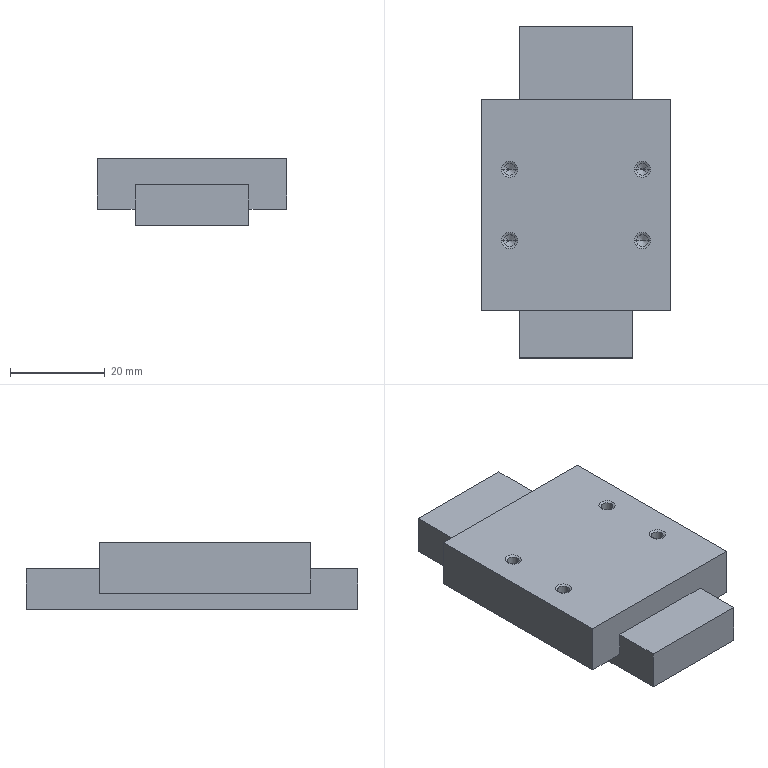Part | NX | 1 solid | 44 faces | box 40 x 70 x 14 mm | volume 27390 mm3 | plane 16 | cone 16 | cylinder 12 | commonest cylinder face diameters 2.5 x8 4.5 x4
STEP:
#1=CARTESIAN_POINT('',(521.985,-261.815,-57.349));
#2=VERTEX_POINT('',#1);
#3=CARTESIAN_POINT('',(526.485,-261.817,-57.349));
#4=VERTEX_POINT('',#3);
#5=CARTESIAN_POINT('',(524.235,-261.816,-57.349));
#6=DIRECTION('',(0.,0.,1.));
#7=DIRECTION('',(1.,-0.0003046,0.));
#8=AXIS2_PLACEMENT_3D('',#5,#6,#7);
#9=CIRCLE('',#8,2.25);
#10=EDGE_CURVE('',#2,#4,#9,.T.);
#11=ORIENTED_EDGE('',*,*,#10,.F.);
#12=CARTESIAN_POINT('',(524.235,-261.816,-57.349));
#13=DIRECTION('',(0.,0.,1.));
#14=DIRECTION('',(1.,-0.0003046,0.));
#15=AXIS2_PLACEMENT_3D('',#12,#13,#14);
#16=CIRCLE('',#15,2.25);
#17=EDGE_CURVE('',#4,#2,#16,.T.);
#18=ORIENTED_EDGE('',*,*,#17,.F.);
#19=EDGE_LOOP('',(#11,#18));
#20=FACE_BOUND('',#19,.T.);
#21=CARTESIAN_POINT('',(520.86,-261.832,-57.349));
#22=DIRECTION('',(0.,0.,1.));
#23=DIRECTION('',(1.,0.,0.));
#24=AXIS2_PLACEMENT_3D('',#21,#22,#23);
#25=PLANE('',#24);
#26=ADVANCED_FACE('',(#20),#25,.F.);
#27=CARTESIAN_POINT('',(536.235,-316.816,-61.349));
#28=VERTEX_POINT('',#27);
#29=CARTESIAN_POINT('',(536.235,-246.816,-61.349));
#30=VERTEX_POINT('',#29);
#31=CARTESIAN_POINT('',(536.235,0.,-61.349));
#32=DIRECTION('',(0.,1.,0.));
#33=VECTOR('',#32,1000.);
#34=LINE('',#31,#33);
#35=EDGE_CURVE('',#28,#30,#34,.T.);
#36=ORIENTED_EDGE('',*,*,#35,.T.);
#37=CARTESIAN_POINT('',(536.235,-246.816,-52.849));
#38=VERTEX_POINT('',#37);
#39=CARTESIAN_POINT('',(536.235,-246.816,0.));
#40=DIRECTION('',(0.,0.,1.));
#41=VECTOR('',#40,1000.);
#42=LINE('',#39,#41);
#43=EDGE_CURVE('',#30,#38,#42,.T.);
#44=ORIENTED_EDGE('',*,*,#43,.T.);
#45=CARTESIAN_POINT('',(536.235,-262.316,-52.849));
#46=VERTEX_POINT('',#45);
#47=CARTESIAN_POINT('',(536.235,0.,-52.849));
#48=DIRECTION('',(0.,1.,0.));
#49=VECTOR('',#48,1000.);
#50=LINE('',#47,#49);
#51=EDGE_CURVE('',#46,#38,#50,.T.);
#52=ORIENTED_EDGE('',*,*,#51,.F.);
#53=CARTESIAN_POINT('',(536.235,-262.316,-57.949));
#54=VERTEX_POINT('',#53);
#55=CARTESIAN_POINT('',(536.235,-262.316,0.));
#56=DIRECTION('',(0.,0.,1.));
#57=VECTOR('',#56,1000.);
#58=LINE('',#55,#57);
#59=EDGE_CURVE('',#54,#46,#58,.T.);
#60=ORIENTED_EDGE('',*,*,#59,.F.);
#61=CARTESIAN_POINT('',(536.235,-306.816,-57.949));
#62=VERTEX_POINT('',#61);
#63=CARTESIAN_POINT('',(536.235,0.,-57.949));
#64=DIRECTION('',(0.,-1.,0.));
#65=VECTOR('',#64,1000.);
#66=LINE('',#63,#65);
#67=EDGE_CURVE('',#54,#62,#66,.T.);
#68=ORIENTED_EDGE('',*,*,#67,.T.);
#69=CARTESIAN_POINT('',(536.235,-306.816,-52.849));
#70=VERTEX_POINT('',#69);
#71=CARTESIAN_POINT('',(536.235,-306.816,0.));
#72=DIRECTION('',(0.,0.,1.));
#73=VECTOR('',#72,1000.);
#74=LINE('',#71,#73);
#75=EDGE_CURVE('',#62,#70,#74,.T.);
#76=ORIENTED_EDGE('',*,*,#75,.T.);
#77=CARTESIAN_POINT('',(536.235,-316.816,-52.849));
#78=VERTEX_POINT('',#77);
#79=CARTESIAN_POINT('',(536.235,0.,-52.849));
#80=DIRECTION('',(0.,1.,0.));
#81=VECTOR('',#80,1000.);
#82=LINE('',#79,#81);
#83=EDGE_CURVE('',#78,#70,#82,.T.);
#84=ORIENTED_EDGE('',*,*,#83,.F.);
#85=CARTESIAN_POINT('',(536.235,-316.816,0.));
#86=DIRECTION('',(0.,0.,-1.));
#87=VECTOR('',#86,1000.);
#88=LINE('',#85,#87);
#89=EDGE_CURVE('',#78,#28,#88,.T.);
#90=ORIENTED_EDGE('',*,*,#89,.T.);
#91=EDGE_LOOP('',(#36,#44,#52,#60,#68,#76,#84,#90));
#92=FACE_BOUND('',#91,.T.);
#93=CARTESIAN_POINT('',(536.235,-306.816,-52.849));
#94=DIRECTION('',(-1.,0.,0.));
#95=DIRECTION('',(0.,1.,0.));
#96=AXIS2_PLACEMENT_3D('',#93,#94,#95);
#97=PLANE('',#96);
#98=ADVANCED_FACE('',(#92),#97,.F.);
#99=CARTESIAN_POINT('',(544.235,-262.316,-47.349));
#100=VERTEX_POINT('',#99);
#101=CARTESIAN_POINT('',(544.235,-306.816,-47.349));
#102=VERTEX_POINT('',#101);
#103=CARTESIAN_POINT('',(544.235,0.,-47.349));
#104=DIRECTION('',(0.,-1.,0.));
#105=VECTOR('',#104,1000.);
#106=LINE('',#103,#105);
#107=EDGE_CURVE('',#100,#102,#106,.T.);
#108=ORIENTED_EDGE('',*,*,#107,.F.);
#109=CARTESIAN_POINT('',(504.235,-262.316,-47.349));
#110=VERTEX_POINT('',#109);
#111=CARTESIAN_POINT('',(0.,-262.316,-47.349));
#112=DIRECTION('',(1.,0.,0.));
#113=VECTOR('',#112,1000.);
#114=LINE('',#111,#113);
#115=EDGE_CURVE('',#110,#100,#114,.T.);
#116=ORIENTED_EDGE('',*,*,#115,.F.);
#117=CARTESIAN_POINT('',(504.235,-306.816,-47.349));
#118=VERTEX_POINT('',#117);
#119=CARTESIAN_POINT('',(504.235,0.,-47.349));
#120=DIRECTION('',(0.,1.,0.));
#121=VECTOR('',#120,1000.);
#122=LINE('',#119,#121);
#123=EDGE_CURVE('',#118,#110,#122,.T.);
#124=ORIENTED_EDGE('',*,*,#123,.F.);
#125=CARTESIAN_POINT('',(0.,-306.816,-47.349));
#126=DIRECTION('',(-1.,0.,0.));
#127=VECTOR('',#126,1000.);
#128=LINE('',#125,#127);
#129=EDGE_CURVE('',#102,#118,#128,.T.);
#130=ORIENTED_EDGE('',*,*,#129,.F.);
#131=EDGE_LOOP('',(#108,#116,#124,#130));
#132=FACE_BOUND('',#131,.T.);
#133=CARTESIAN_POINT('',(511.935,-277.066,-47.349));
#134=VERTEX_POINT('',#133);
#135=CARTESIAN_POINT('',(508.535,-277.066,-47.349));
#136=VERTEX_POINT('',#135);
#137=CARTESIAN_POINT('',(510.235,-277.066,-47.349));
#138=DIRECTION('',(0.,0.,1.));
#139=DIRECTION('',(1.,0.,0.));
#140=AXIS2_PLACEMENT_3D('',#137,#138,#139);
#141=CIRCLE('',#140,1.7);
#142=EDGE_CURVE('',#134,#136,#141,.T.);
#143=ORIENTED_EDGE('',*,*,#142,.F.);
#144=CARTESIAN_POINT('',(510.235,-277.066,-47.349));
#145=DIRECTION('',(0.,0.,1.));
#146=DIRECTION('',(1.,0.,0.));
#147=AXIS2_PLACEMENT_3D('',#144,#145,#146);
#148=CIRCLE('',#147,1.7);
#149=EDGE_CURVE('',#136,#134,#148,.T.);
#150=ORIENTED_EDGE('',*,*,#149,.F.);
#151=EDGE_LOOP('',(#143,#150));
#152=FACE_BOUND('',#151,.T.);
#153=CARTESIAN_POINT('',(539.935,-277.066,-47.349));
#154=VERTEX_POINT('',#153);
#155=CARTESIAN_POINT('',(536.535,-277.066,-47.349));
#156=VERTEX_POINT('',#155);
#157=CARTESIAN_POINT('',(538.235,-277.066,-47.349));
#158=DIRECTION('',(0.,0.,1.));
#159=DIRECTION('',(1.,0.,0.));
#160=AXIS2_PLACEMENT_3D('',#157,#158,#159);
#161=CIRCLE('',#160,1.7);
#162=EDGE_CURVE('',#154,#156,#161,.T.);
#163=ORIENTED_EDGE('',*,*,#162,.F.);
#164=CARTESIAN_POINT('',(538.235,-277.066,-47.349));
#165=DIRECTION('',(0.,0.,1.));
#166=DIRECTION('',(1.,0.,0.));
#167=AXIS2_PLACEMENT_3D('',#164,#165,#166);
#168=CIRCLE('',#167,1.7);
#169=EDGE_CURVE('',#156,#154,#168,.T.);
#170=ORIENTED_EDGE('',*,*,#169,.F.);
#171=EDGE_LOOP('',(#163,#170));
#172=FACE_BOUND('',#171,.T.);
#173=CARTESIAN_POINT('',(508.535,-292.066,-47.349));
#174=VERTEX_POINT('',#173);
#175=CARTESIAN_POINT('',(511.935,-292.066,-47.349));
#176=VERTEX_POINT('',#175);
#177=CARTESIAN_POINT('',(510.235,-292.066,-47.349));
#178=DIRECTION('',(0.,0.,1.));
#179=DIRECTION('',(1.,0.,0.));
#180=AXIS2_PLACEMENT_3D('',#177,#178,#179);
#181=CIRCLE('',#180,1.7);
#182=EDGE_CURVE('',#174,#176,#181,.T.);
#183=ORIENTED_EDGE('',*,*,#182,.F.);
#184=CARTESIAN_POINT('',(510.235,-292.066,-47.349));
#185=DIRECTION('',(0.,0.,1.));
#186=DIRECTION('',(1.,0.,0.));
#187=AXIS2_PLACEMENT_3D('',#184,#185,#186);
#188=CIRCLE('',#187,1.7);
#189=EDGE_CURVE('',#176,#174,#188,.T.);
#190=ORIENTED_EDGE('',*,*,#189,.F.);
#191=EDGE_LOOP('',(#183,#190));
#192=FACE_BOUND('',#191,.T.);
#193=CARTESIAN_POINT('',(536.535,-292.066,-47.349));
#194=VERTEX_POINT('',#193);
#195=CARTESIAN_POINT('',(539.935,-292.066,-47.349));
#196=VERTEX_POINT('',#195);
#197=CARTESIAN_POINT('',(538.235,-292.066,-47.349));
#198=DIRECTION('',(0.,0.,1.));
#199=DIRECTION('',(1.,0.,0.));
#200=AXIS2_PLACEMENT_3D('',#197,#198,#199);
#201=CIRCLE('',#200,1.7);
#202=EDGE_CURVE('',#194,#196,#201,.T.);
#203=ORIENTED_EDGE('',*,*,#202,.F.);
#204=CARTESIAN_POINT('',(538.235,-292.066,-47.349));
#205=DIRECTION('',(0.,0.,1.));
#206=DIRECTION('',(1.,0.,0.));
#207=AXIS2_PLACEMENT_3D('',#204,#205,#206);
#208=CIRCLE('',#207,1.7);
#209=EDGE_CURVE('',#196,#194,#208,.T.);
#210=ORIENTED_EDGE('',*,*,#209,.F.);
#211=EDGE_LOOP('',(#203,#210));
#212=FACE_BOUND('',#211,.T.);
#213=CARTESIAN_POINT('',(504.235,-306.816,-47.349));
#214=DIRECTION('',(0.,0.,-1.));
#215=DIRECTION('',(-1.,0.,0.));
#216=AXIS2_PLACEMENT_3D('',#213,#214,#215);
#217=PLANE('',#216);
#218=ADVANCED_FACE('',(#132,#152,#172,#192,#212),#217,.F.);
#219=CARTESIAN_POINT('',(512.235,-316.816,-52.849));
#220=VERTEX_POINT('',#219);
#221=CARTESIAN_POINT('',(512.235,-306.816,-52.849));
#222=VERTEX_POINT('',#221);
#223=CARTESIAN_POINT('',(512.235,0.,-52.849));
#224=DIRECTION('',(0.,1.,0.));
#225=VECTOR('',#224,1000.);
#226=LINE('',#223,#225);
#227=EDGE_CURVE('',#220,#222,#226,.T.);
#228=ORIENTED_EDGE('',*,*,#227,.T.);
#229=CARTESIAN_POINT('',(512.235,-306.816,-57.949));
#230=VERTEX_POINT('',#229);
#231=CARTESIAN_POINT('',(512.235,-306.816,0.));
#232=DIRECTION('',(0.,0.,-1.));
#233=VECTOR('',#232,1000.);
#234=LINE('',#231,#233);
#235=EDGE_CURVE('',#222,#230,#234,.T.);
#236=ORIENTED_EDGE('',*,*,#235,.T.);
#237=CARTESIAN_POINT('',(512.235,-262.316,-57.949));
#238=VERTEX_POINT('',#237);
#239=CARTESIAN_POINT('',(512.235,0.,-57.949));
#240=DIRECTION('',(0.,1.,0.));
#241=VECTOR('',#240,1000.);
#242=LINE('',#239,#241);
#243=EDGE_CURVE('',#230,#238,#242,.T.);
#244=ORIENTED_EDGE('',*,*,#243,.T.);
#245=CARTESIAN_POINT('',(512.235,-262.316,-52.849));
#246=VERTEX_POINT('',#245);
#247=CARTESIAN_POINT('',(512.235,-262.316,0.));
#248=DIRECTION('',(0.,0.,-1.));
#249=VECTOR('',#248,1000.);
#250=LINE('',#247,#249);
#251=EDGE_CURVE('',#246,#238,#250,.T.);
#252=ORIENTED_EDGE('',*,*,#251,.F.);
#253=CARTESIAN_POINT('',(512.235,-246.816,-52.849));
#254=VERTEX_POINT('',#253);
#255=CARTESIAN_POINT('',(512.235,0.,-52.849));
#256=DIRECTION('',(0.,-1.,0.));
#257=VECTOR('',#256,1000.);
#258=LINE('',#255,#257);
#259=EDGE_CURVE('',#254,#246,#258,.T.);
#260=ORIENTED_EDGE('',*,*,#259,.F.);
#261=CARTESIAN_POINT('',(512.235,-246.816,-61.349));
#262=VERTEX_POINT('',#261);
#263=CARTESIAN_POINT('',(512.235,-246.816,0.));
#264=DIRECTION('',(0.,0.,-1.));
#265=VECTOR('',#264,1000.);
#266=LINE('',#263,#265);
#267=EDGE_CURVE('',#254,#262,#266,.T.);
#268=ORIENTED_EDGE('',*,*,#267,.T.);
#269=CARTESIAN_POINT('',(512.235,-316.816,-61.349));
#270=VERTEX_POINT('',#269);
#271=CARTESIAN_POINT('',(512.235,0.,-61.349));
#272=DIRECTION('',(0.,-1.,0.));
#273=VECTOR('',#272,1000.);
#274=LINE('',#271,#273);
#275=EDGE_CURVE('',#262,#270,#274,.T.);
#276=ORIENTED_EDGE('',*,*,#275,.T.);
#277=CARTESIAN_POINT('',(512.235,-316.816,0.));
#278=DIRECTION('',(0.,0.,1.));
#279=VECTOR('',#278,1000.);
#280=LINE('',#277,#279);
#281=EDGE_CURVE('',#270,#220,#280,.T.);
#282=ORIENTED_EDGE('',*,*,#281,.T.);
#283=EDGE_LOOP('',(#228,#236,#244,#252,#260,#268,#276,#282));
#284=FACE_BOUND('',#283,.T.);
#285=CARTESIAN_POINT('',(512.235,-306.816,-61.349));
#286=DIRECTION('',(1.,0.,0.));
#287=DIRECTION('',(0.,0.,-1.));
#288=AXIS2_PLACEMENT_3D('',#285,#286,#287);
#289=PLANE('',#288);
#290=ADVANCED_FACE('',(#284),#289,.F.);
#291=ORIENTED_EDGE('',*,*,#83,.T.);
#292=CARTESIAN_POINT('',(0.,-306.816,-52.849));
#293=DIRECTION('',(-1.,0.,0.));
#294=VECTOR('',#293,1000.);
#295=LINE('',#292,#294);
#296=EDGE_CURVE('',#70,#222,#295,.T.);
#297=ORIENTED_EDGE('',*,*,#296,.T.);
#298=ORIENTED_EDGE('',*,*,#227,.F.);
#299=CARTESIAN_POINT('',(0.,-316.816,-52.849));
#300=DIRECTION('',(1.,0.,0.));
#301=VECTOR('',#300,1000.);
#302=LINE('',#299,#301);
#303=EDGE_CURVE('',#220,#78,#302,.T.);
#304=ORIENTED_EDGE('',*,*,#303,.T.);
#305=EDGE_LOOP('',(#291,#297,#298,#304));
#306=FACE_BOUND('',#305,.T.);
#307=CARTESIAN_POINT('',(512.235,-306.816,-52.849));
#308=DIRECTION('',(0.,0.,-1.));
#309=DIRECTION('',(-1.,0.,0.));
#310=AXIS2_PLACEMENT_3D('',#307,#308,#309);
#311=PLANE('',#310);
#312=ADVANCED_FACE('',(#306),#311,.F.);
#313=ORIENTED_EDGE('',*,*,#67,.F.);
#314=CARTESIAN_POINT('',(544.235,-262.316,-57.949));
#315=VERTEX_POINT('',#314);
#316=CARTESIAN_POINT('',(0.,-262.316,-57.949));
#317=DIRECTION('',(1.,0.,0.));
#318=VECTOR('',#317,1000.);
#319=LINE('',#316,#318);
#320=EDGE_CURVE('',#54,#315,#319,.T.);
#321=ORIENTED_EDGE('',*,*,#320,.T.);
#322=CARTESIAN_POINT('',(544.235,-306.816,-57.949));
#323=VERTEX_POINT('',#322);
#324=CARTESIAN_POINT('',(544.235,0.,-57.949));
#325=DIRECTION('',(0.,1.,0.));
#326=VECTOR('',#325,1000.);
#327=LINE('',#324,#326);
#328=EDGE_CURVE('',#323,#315,#327,.T.);
#329=ORIENTED_EDGE('',*,*,#328,.F.);
#330=CARTESIAN_POINT('',(0.,-306.816,-57.949));
#331=DIRECTION('',(1.,0.,0.));
#332=VECTOR('',#331,1000.);
#333=LINE('',#330,#332);
#334=EDGE_CURVE('',#62,#323,#333,.T.);
#335=ORIENTED_EDGE('',*,*,#334,.F.);
#336=EDGE_LOOP('',(#313,#321,#329,#335));
#337=FACE_BOUND('',#336,.T.);
#338=CARTESIAN_POINT('',(544.235,-306.816,-57.949));
#339=DIRECTION('',(0.,0.,1.));
#340=DIRECTION('',(1.,0.,0.));
#341=AXIS2_PLACEMENT_3D('',#338,#339,#340);
#342=PLANE('',#341);
#343=ADVANCED_FACE('',(#337),#342,.F.);
#344=CARTESIAN_POINT('',(504.235,-262.316,-57.949));
#345=VERTEX_POINT('',#344);
#346=CARTESIAN_POINT('',(0.,-262.316,-57.949));
#347=DIRECTION('',(-1.,0.,0.));
#348=VECTOR('',#347,1000.);
#349=LINE('',#346,#348);
#350=EDGE_CURVE('',#238,#345,#349,.T.);
#351=ORIENTED_EDGE('',*,*,#350,.T.);
#352=CARTESIAN_POINT('',(504.235,-262.316,0.));
#353=DIRECTION('',(0.,0.,1.));
#354=VECTOR('',#353,1000.);
#355=LINE('',#352,#354);
#356=EDGE_CURVE('',#345,#110,#355,.T.);
#357=ORIENTED_EDGE('',*,*,#356,.T.);
#358=ORIENTED_EDGE('',*,*,#115,.T.);
#359=CARTESIAN_POINT('',(544.235,-262.316,0.));
#360=DIRECTION('',(0.,0.,-1.));
#361=VECTOR('',#360,1000.);
#362=LINE('',#359,#361);
#363=EDGE_CURVE('',#100,#315,#362,.T.);
#364=ORIENTED_EDGE('',*,*,#363,.T.);
#365=ORIENTED_EDGE('',*,*,#320,.F.);
#366=ORIENTED_EDGE('',*,*,#59,.T.);
#367=CARTESIAN_POINT('',(0.,-262.316,-52.849));
#368=DIRECTION('',(1.,0.,0.));
#369=VECTOR('',#368,1000.);
#370=LINE('',#367,#369);
#371=EDGE_CURVE('',#246,#46,#370,.T.);
#372=ORIENTED_EDGE('',*,*,#371,.F.);
#373=ORIENTED_EDGE('',*,*,#251,.T.);
#374=EDGE_LOOP('',(#351,#357,#358,#364,#365,#366,#372,#373));
#375=FACE_BOUND('',#374,.T.);
#376=CARTESIAN_POINT('',(492.609,-262.316,-65.209));
#377=DIRECTION('',(0.,1.,0.));
#378=DIRECTION('',(1.,0.,0.));
#379=AXIS2_PLACEMENT_3D('',#376,#377,#378);
#380=PLANE('',#379);
#381=ADVANCED_FACE('',(#375),#380,.T.);
#382=CARTESIAN_POINT('',(504.235,-306.816,-57.949));
#383=VERTEX_POINT('',#382);
#384=CARTESIAN_POINT('',(504.235,0.,-57.949));
#385=DIRECTION('',(0.,-1.,0.));
#386=VECTOR('',#385,1000.);
#387=LINE('',#384,#386);
#388=EDGE_CURVE('',#345,#383,#387,.T.);
#389=ORIENTED_EDGE('',*,*,#388,.F.);
#390=ORIENTED_EDGE('',*,*,#350,.F.);
#391=ORIENTED_EDGE('',*,*,#243,.F.);
#392=CARTESIAN_POINT('',(0.,-306.816,-57.949));
#393=DIRECTION('',(1.,0.,0.));
#394=VECTOR('',#393,1000.);
#395=LINE('',#392,#394);
#396=EDGE_CURVE('',#383,#230,#395,.T.);
#397=ORIENTED_EDGE('',*,*,#396,.F.);
#398=EDGE_LOOP('',(#389,#390,#391,#397));
#399=FACE_BOUND('',#398,.T.);
#400=CARTESIAN_POINT('',(512.235,-306.816,-57.949));
#401=DIRECTION('',(0.,0.,1.));
#402=DIRECTION('',(1.,0.,0.));
#403=AXIS2_PLACEMENT_3D('',#400,#401,#402);
#404=PLANE('',#403);
#405=ADVANCED_FACE('',(#399),#404,.F.);
#406=ORIENTED_EDGE('',*,*,#235,.F.);
#407=ORIENTED_EDGE('',*,*,#296,.F.);
#408=ORIENTED_EDGE('',*,*,#75,.F.);
#409=ORIENTED_EDGE('',*,*,#334,.T.);
#410=CARTESIAN_POINT('',(544.235,-306.816,0.));
#411=DIRECTION('',(0.,0.,-1.));
#412=VECTOR('',#411,1000.);
#413=LINE('',#410,#412);
#414=EDGE_CURVE('',#102,#323,#413,.T.);
#415=ORIENTED_EDGE('',*,*,#414,.F.);
#416=ORIENTED_EDGE('',*,*,#129,.T.);
#417=CARTESIAN_POINT('',(504.235,-306.816,0.));
#418=DIRECTION('',(0.,0.,-1.));
#419=VECTOR('',#418,1000.);
#420=LINE('',#417,#419);
#421=EDGE_CURVE('',#118,#383,#420,.T.);
#422=ORIENTED_EDGE('',*,*,#421,.T.);
#423=ORIENTED_EDGE('',*,*,#396,.T.);
#424=EDGE_LOOP('',(#406,#407,#408,#409,#415,#416,#422,#423));
#425=FACE_BOUND('',#424,.T.);
#426=CARTESIAN_POINT('',(492.609,-306.816,-65.209));
#427=DIRECTION('',(0.,1.,0.));
#428=DIRECTION('',(1.,0.,0.));
#429=AXIS2_PLACEMENT_3D('',#426,#427,#428);
#430=PLANE('',#429);
#431=ADVANCED_FACE('',(#425),#430,.F.);
#432=ORIENTED_EDGE('',*,*,#51,.T.);
#433=CARTESIAN_POINT('',(0.,-246.816,-52.849));
#434=DIRECTION('',(1.,0.,0.));
#435=VECTOR('',#434,1000.);
#436=LINE('',#433,#435);
#437=EDGE_CURVE('',#254,#38,#436,.T.);
#438=ORIENTED_EDGE('',*,*,#437,.F.);
#439=ORIENTED_EDGE('',*,*,#259,.T.);
#440=ORIENTED_EDGE('',*,*,#371,.T.);
#441=EDGE_LOOP('',(#432,#438,#439,#440));
#442=FACE_BOUND('',#441,.T.);
#443=CARTESIAN_POINT('',(520.86,-251.832,-52.849));
#444=DIRECTION('',(0.,0.,1.));
#445=DIRECTION('',(1.,0.,0.));
#446=AXIS2_PLACEMENT_3D('',#443,#444,#445);
#447=PLANE('',#446);
#448=ADVANCED_FACE('',(#442),#447,.T.);
#449=ORIENTED_EDGE('',*,*,#123,.T.);
#450=ORIENTED_EDGE('',*,*,#356,.F.);
#451=ORIENTED_EDGE('',*,*,#388,.T.);
#452=ORIENTED_EDGE('',*,*,#421,.F.);
#453=EDGE_LOOP('',(#449,#450,#451,#452));
#454=FACE_BOUND('',#453,.T.);
#455=CARTESIAN_POINT('',(504.235,-306.816,-57.949));
#456=DIRECTION('',(1.,0.,0.));
#457=DIRECTION('',(0.,0.,-1.));
#458=AXIS2_PLACEMENT_3D('',#455,#456,#457);
#459=PLANE('',#458);
#460=ADVANCED_FACE('',(#454),#459,.F.);
#461=ORIENTED_EDGE('',*,*,#328,.T.);
#462=ORIENTED_EDGE('',*,*,#363,.F.);
#463=ORIENTED_EDGE('',*,*,#107,.T.);
#464=ORIENTED_EDGE('',*,*,#414,.T.);
#465=EDGE_LOOP('',(#461,#462,#463,#464));
#466=FACE_BOUND('',#465,.T.);
#467=CARTESIAN_POINT('',(544.235,-306.816,-47.349));
#468=DIRECTION('',(-1.,0.,0.));
#469=DIRECTION('',(0.,1.,0.));
#470=AXIS2_PLACEMENT_3D('',#467,#468,#469);
#471=PLANE('',#470);
#472=ADVANCED_FACE('',(#466),#471,.F.);
#473=CARTESIAN_POINT('',(508.985,-277.066,-56.349));
#474=VERTEX_POINT('',#473);
#475=CARTESIAN_POINT('',(511.485,-277.066,-56.349));
#476=VERTEX_POINT('',#475);
#477=CARTESIAN_POINT('',(510.235,-277.066,-56.349));
#478=DIRECTION('',(0.,0.,-1.));
#479=DIRECTION('',(-1.,0.,0.));
#480=AXIS2_PLACEMENT_3D('',#477,#478,#479);
#481=CIRCLE('',#480,1.25);
#482=EDGE_CURVE('',#474,#476,#481,.T.);
#483=ORIENTED_EDGE('',*,*,#482,.T.);
#484=CARTESIAN_POINT('',(511.485,-277.066,-47.608));
#485=VERTEX_POINT('',#484);
#486=CARTESIAN_POINT('',(511.485,-277.066,-50.349));
#487=DIRECTION('',(0.,0.,1.));
#488=VECTOR('',#487,1000.);
#489=LINE('',#486,#488);
#490=EDGE_CURVE('',#485,#476,#489,.F.);
#491=ORIENTED_EDGE('',*,*,#490,.F.);
#492=CARTESIAN_POINT('',(508.985,-277.066,-47.608));
#493=VERTEX_POINT('',#492);
#494=CARTESIAN_POINT('',(510.235,-277.066,-47.608));
#495=DIRECTION('',(0.,0.,1.));
#496=DIRECTION('',(1.,0.,0.));
#497=AXIS2_PLACEMENT_3D('',#494,#495,#496);
#498=CIRCLE('',#497,1.25);
#499=EDGE_CURVE('',#485,#493,#498,.T.);
#500=ORIENTED_EDGE('',*,*,#499,.T.);
#501=CARTESIAN_POINT('',(508.985,-277.066,-50.349));
#502=DIRECTION('',(0.,0.,1.));
#503=VECTOR('',#502,1000.);
#504=LINE('',#501,#503);
#505=EDGE_CURVE('',#493,#474,#504,.F.);
#506=ORIENTED_EDGE('',*,*,#505,.T.);
#507=EDGE_LOOP('',(#483,#491,#500,#506));
#508=FACE_BOUND('',#507,.T.);
#509=CARTESIAN_POINT('',(510.235,-277.066,-50.349));
#510=DIRECTION('',(0.,0.,1.));
#511=DIRECTION('',(-1.,0.,0.));
#512=AXIS2_PLACEMENT_3D('',#509,#510,#511);
#513=CYLINDRICAL_SURFACE('',#512,1.25);
#514=ADVANCED_FACE('',(#508),#513,.F.);
#515=ORIENTED_EDGE('',*,*,#162,.T.);
#516=CARTESIAN_POINT('',(536.985,-277.066,-47.608));
#517=VERTEX_POINT('',#516);
#518=CARTESIAN_POINT('',(536.535,-277.066,-47.349));
#519=DIRECTION('',(-0.866,0.,0.5));
#520=VECTOR('',#519,1000.);
#521=LINE('',#518,#520);
#522=EDGE_CURVE('',#517,#156,#521,.T.);
#523=ORIENTED_EDGE('',*,*,#522,.F.);
#524=CARTESIAN_POINT('',(539.485,-277.066,-47.608));
#525=VERTEX_POINT('',#524);
#526=CARTESIAN_POINT('',(538.235,-277.066,-47.608));
#527=DIRECTION('',(0.,0.,1.));
#528=DIRECTION('',(1.,0.,0.));
#529=AXIS2_PLACEMENT_3D('',#526,#527,#528);
#530=CIRCLE('',#529,1.25);
#531=EDGE_CURVE('',#525,#517,#530,.T.);
#532=ORIENTED_EDGE('',*,*,#531,.F.);
#533=CARTESIAN_POINT('',(539.935,-277.066,-47.349));
#534=DIRECTION('',(0.866,0.,0.5));
#535=VECTOR('',#534,1000.);
#536=LINE('',#533,#535);
#537=EDGE_CURVE('',#525,#154,#536,.T.);
#538=ORIENTED_EDGE('',*,*,#537,.T.);
#539=EDGE_LOOP('',(#515,#523,#532,#538));
#540=FACE_BOUND('',#539,.T.);
#541=CARTESIAN_POINT('',(538.235,-277.066,-47.349));
#542=DIRECTION('',(0.,0.,1.));
#543=DIRECTION('',(1.,0.,0.));
#544=AXIS2_PLACEMENT_3D('',#541,#542,#543);
#545=CONICAL_SURFACE('',#544,1.7,1.047);
#546=ADVANCED_FACE('',(#540),#545,.F.);
#547=CARTESIAN_POINT('',(521.985,-301.816,-57.349));
#548=VERTEX_POINT('',#547);
#549=CARTESIAN_POINT('',(526.485,-301.816,-57.349));
#550=VERTEX_POINT('',#549);
#551=CARTESIAN_POINT('',(524.235,-301.816,-57.349));
#552=DIRECTION('',(0.,0.,-1.));
#553=DIRECTION('',(1.,0.,0.));
#554=AXIS2_PLACEMENT_3D('',#551,#552,#553);
#555=CIRCLE('',#554,2.25);
#556=EDGE_CURVE('',#548,#550,#555,.T.);
#557=ORIENTED_EDGE('',*,*,#556,.T.);
#558=CARTESIAN_POINT('',(524.235,-301.816,-57.349));
#559=DIRECTION('',(0.,0.,-1.));
#560=DIRECTION('',(1.,0.,0.));
#561=AXIS2_PLACEMENT_3D('',#558,#559,#560);
#562=CIRCLE('',#561,2.25);
#563=EDGE_CURVE('',#550,#548,#562,.T.);
#564=ORIENTED_EDGE('',*,*,#563,.T.);
#565=EDGE_LOOP('',(#557,#564));
#566=FACE_BOUND('',#565,.T.);
#567=CARTESIAN_POINT('',(522.543,-287.947,-57.349));
#568=DIRECTION('',(0.,0.,-1.));
#569=DIRECTION('',(-1.,0.,0.));
#570=AXIS2_PLACEMENT_3D('',#567,#568,#569);
#571=PLANE('',#570);
#572=ADVANCED_FACE('',(#566),#571,.T.);
#573=CARTESIAN_POINT('',(510.235,-277.066,-57.1));
#574=VERTEX_POINT('',#573);
#575=CARTESIAN_POINT('',(508.985,-277.066,-56.349));
#576=DIRECTION('',(-0.8572,0.,0.515));
#577=VECTOR('',#576,1000.);
#578=LINE('',#575,#577);
#579=EDGE_CURVE('',#474,#574,#578,.F.);
#580=ORIENTED_EDGE('',*,*,#579,.F.);
#581=CARTESIAN_POINT('',(510.235,-277.066,-56.349));
#582=DIRECTION('',(0.,0.,-1.));
#583=DIRECTION('',(-1.,0.,0.));
#584=AXIS2_PLACEMENT_3D('',#581,#582,#583);
#585=CIRCLE('',#584,1.25);
#586=EDGE_CURVE('',#476,#474,#585,.T.);
#587=ORIENTED_EDGE('',*,*,#586,.F.);
#588=CARTESIAN_POINT('',(511.485,-277.066,-56.349));
#589=DIRECTION('',(0.8572,0.,0.515));
#590=VECTOR('',#589,1000.);
#591=LINE('',#588,#590);
#592=EDGE_CURVE('',#476,#574,#591,.F.);
#593=ORIENTED_EDGE('',*,*,#592,.T.);
#594=EDGE_LOOP('',(#580,#587,#593));
#595=FACE_BOUND('',#594,.T.);
#596=CARTESIAN_POINT('',(510.235,-277.066,-56.349));
#597=DIRECTION('',(0.,0.,1.));
#598=DIRECTION('',(1.,0.,0.));
#599=AXIS2_PLACEMENT_3D('',#596,#597,#598);
#600=CONICAL_SURFACE('',#599,1.25,1.03);
#601=ADVANCED_FACE('',(#595),#600,.F.);
#602=CARTESIAN_POINT('',(511.485,-292.066,-47.608));
#603=VERTEX_POINT('',#602);
#604=CARTESIAN_POINT('',(508.985,-292.066,-47.608));
#605=VERTEX_POINT('',#604);
#606=CARTESIAN_POINT('',(510.235,-292.066,-47.608));
#607=DIRECTION('',(0.,0.,1.));
#608=DIRECTION('',(1.,0.,0.));
#609=AXIS2_PLACEMENT_3D('',#606,#607,#608);
#610=CIRCLE('',#609,1.25);
#611=EDGE_CURVE('',#603,#605,#610,.T.);
#612=ORIENTED_EDGE('',*,*,#611,.T.);
#613=CARTESIAN_POINT('',(508.985,-292.066,-56.349));
#614=VERTEX_POINT('',#613);
#615=CARTESIAN_POINT('',(508.985,-292.066,-50.349));
#616=DIRECTION('',(0.,0.,1.));
#617=VECTOR('',#616,1000.);
#618=LINE('',#615,#617);
#619=EDGE_CURVE('',#605,#614,#618,.F.);
#620=ORIENTED_EDGE('',*,*,#619,.T.);
#621=CARTESIAN_POINT('',(511.485,-292.066,-56.349));
#622=VERTEX_POINT('',#621);
#623=CARTESIAN_POINT('',(510.235,-292.066,-56.349));
#624=DIRECTION('',(0.,0.,-1.));
#625=DIRECTION('',(-1.,0.,0.));
#626=AXIS2_PLACEMENT_3D('',#623,#624,#625);
#627=CIRCLE('',#626,1.25);
#628=EDGE_CURVE('',#614,#622,#627,.T.);
#629=ORIENTED_EDGE('',*,*,#628,.T.);
#630=CARTESIAN_POINT('',(511.485,-292.066,-50.349));
#631=DIRECTION('',(0.,0.,1.));
#632=VECTOR('',#631,1000.);
#633=LINE('',#630,#632);
#634=EDGE_CURVE('',#603,#622,#633,.F.);
#635=ORIENTED_EDGE('',*,*,#634,.F.);
#636=EDGE_LOOP('',(#612,#620,#629,#635));
#637=FACE_BOUND('',#636,.T.);
#638=CARTESIAN_POINT('',(510.235,-292.066,-50.349));
#639=DIRECTION('',(0.,0.,1.));
#640=DIRECTION('',(-1.,0.,0.));
#641=AXIS2_PLACEMENT_3D('',#638,#639,#640);
#642=CYLINDRICAL_SURFACE('',#641,1.25);
#643=ADVANCED_FACE('',(#637),#642,.F.);
#644=ORIENTED_EDGE('',*,*,#499,.F.);
#645=CARTESIAN_POINT('',(511.485,-277.066,-47.608));
#646=DIRECTION('',(0.866,0.,0.5));
#647=VECTOR('',#646,1000.);
#648=LINE('',#645,#647);
#649=EDGE_CURVE('',#485,#134,#648,.T.);
#650=ORIENTED_EDGE('',*,*,#649,.T.);
#651=ORIENTED_EDGE('',*,*,#142,.T.);
#652=CARTESIAN_POINT('',(508.985,-277.066,-47.608));
#653=DIRECTION('',(-0.866,0.,0.5));
#654=VECTOR('',#653,1000.);
#655=LINE('',#652,#654);
#656=EDGE_CURVE('',#493,#136,#655,.T.);
#657=ORIENTED_EDGE('',*,*,#656,.F.);
#658=EDGE_LOOP('',(#644,#650,#651,#657));
#659=FACE_BOUND('',#658,.T.);
#660=CARTESIAN_POINT('',(510.235,-277.066,-47.608));
#661=DIRECTION('',(0.,0.,1.));
#662=DIRECTION('',(1.,0.,0.));
#663=AXIS2_PLACEMENT_3D('',#660,#661,#662);
#664=CONICAL_SURFACE('',#663,1.25,1.047);
#665=ADVANCED_FACE('',(#659),#664,.F.);
#666=ORIENTED_EDGE('',*,*,#556,.F.);
#667=CARTESIAN_POINT('',(521.985,-301.816,-61.349));
#668=VERTEX_POINT('',#667);
#669=CARTESIAN_POINT('',(521.985,-301.816,-61.349));
#670=DIRECTION('',(0.,0.,-1.));
#671=VECTOR('',#670,1000.);
#672=LINE('',#669,#671);
#673=EDGE_CURVE('',#668,#548,#672,.F.);
#674=ORIENTED_EDGE('',*,*,#673,.F.);
#675=CARTESIAN_POINT('',(526.485,-301.816,-61.349));
#676=VERTEX_POINT('',#675);
#677=CARTESIAN_POINT('',(524.235,-301.816,-61.349));
#678=DIRECTION('',(0.,0.,-1.));
#679=DIRECTION('',(1.,0.,0.));
#680=AXIS2_PLACEMENT_3D('',#677,#678,#679);
#681=CIRCLE('',#680,2.25);
#682=EDGE_CURVE('',#668,#676,#681,.T.);
#683=ORIENTED_EDGE('',*,*,#682,.T.);
#684=CARTESIAN_POINT('',(526.485,-301.816,-61.349));
#685=DIRECTION('',(0.,0.,-1.));
#686=VECTOR('',#685,1000.);
#687=LINE('',#684,#686);
#688=EDGE_CURVE('',#676,#550,#687,.F.);
#689=ORIENTED_EDGE('',*,*,#688,.T.);
#690=EDGE_LOOP('',(#666,#674,#683,#689));
#691=FACE_BOUND('',#690,.T.);
#692=CARTESIAN_POINT('',(524.235,-301.816,-61.349));
#693=DIRECTION('',(0.,0.,-1.));
#694=DIRECTION('',(1.,0.,0.));
#695=AXIS2_PLACEMENT_3D('',#692,#693,#694);
#696=CYLINDRICAL_SURFACE('',#695,2.25);
#697=ADVANCED_FACE('',(#691),#696,.F.);
#698=CARTESIAN_POINT('',(510.235,-292.066,-57.1));
#699=VERTEX_POINT('',#698);
#700=CARTESIAN_POINT('',(508.985,-292.066,-56.349));
#701=DIRECTION('',(-0.8572,0.,0.515));
#702=VECTOR('',#701,1000.);
#703=LINE('',#700,#702);
#704=EDGE_CURVE('',#614,#699,#703,.F.);
#705=ORIENTED_EDGE('',*,*,#704,.F.);
#706=CARTESIAN_POINT('',(510.235,-292.066,-56.349));
#707=DIRECTION('',(0.,0.,-1.));
#708=DIRECTION('',(-1.,0.,0.));
#709=AXIS2_PLACEMENT_3D('',#706,#707,#708);
#710=CIRCLE('',#709,1.25);
#711=EDGE_CURVE('',#622,#614,#710,.T.);
#712=ORIENTED_EDGE('',*,*,#711,.F.);
#713=CARTESIAN_POINT('',(511.485,-292.066,-56.349));
#714=DIRECTION('',(0.8572,0.,0.515));
#715=VECTOR('',#714,1000.);
#716=LINE('',#713,#715);
#717=EDGE_CURVE('',#622,#699,#716,.F.);
#718=ORIENTED_EDGE('',*,*,#717,.T.);
#719=EDGE_LOOP('',(#705,#712,#718));
#720=FACE_BOUND('',#719,.T.);
#721=CARTESIAN_POINT('',(510.235,-292.066,-56.349));
#722=DIRECTION('',(0.,0.,1.));
#723=DIRECTION('',(1.,0.,0.));
#724=AXIS2_PLACEMENT_3D('',#721,#722,#723);
#725=CONICAL_SURFACE('',#724,1.25,1.03);
#726=ADVANCED_FACE('',(#720),#725,.F.);
#727=CARTESIAN_POINT('',(536.985,-292.066,-56.349));
#728=VERTEX_POINT('',#727);
#729=CARTESIAN_POINT('',(539.485,-292.066,-56.349));
#730=VERTEX_POINT('',#729);
#731=CARTESIAN_POINT('',(538.235,-292.066,-56.349));
#732=DIRECTION('',(0.,0.,-1.));
#733=DIRECTION('',(-1.,0.,0.));
#734=AXIS2_PLACEMENT_3D('',#731,#732,#733);
#735=CIRCLE('',#734,1.25);
#736=EDGE_CURVE('',#728,#730,#735,.T.);
#737=ORIENTED_EDGE('',*,*,#736,.T.);
#738=CARTESIAN_POINT('',(539.485,-292.066,-47.608));
#739=VERTEX_POINT('',#738);
#740=CARTESIAN_POINT('',(539.485,-292.066,-50.349));
#741=DIRECTION('',(0.,0.,1.));
#742=VECTOR('',#741,1000.);
#743=LINE('',#740,#742);
#744=EDGE_CURVE('',#739,#730,#743,.F.);
#745=ORIENTED_EDGE('',*,*,#744,.F.);
#746=CARTESIAN_POINT('',(536.985,-292.066,-47.608));
#747=VERTEX_POINT('',#746);
#748=CARTESIAN_POINT('',(538.235,-292.066,-47.608));
#749=DIRECTION('',(0.,0.,1.));
#750=DIRECTION('',(1.,0.,0.));
#751=AXIS2_PLACEMENT_3D('',#748,#749,#750);
#752=CIRCLE('',#751,1.25);
#753=EDGE_CURVE('',#739,#747,#752,.T.);
#754=ORIENTED_EDGE('',*,*,#753,.T.);
#755=CARTESIAN_POINT('',(536.985,-292.066,-50.349));
#756=DIRECTION('',(0.,0.,1.));
#757=VECTOR('',#756,1000.);
#758=LINE('',#755,#757);
#759=EDGE_CURVE('',#747,#728,#758,.F.);
#760=ORIENTED_EDGE('',*,*,#759,.T.);
#761=EDGE_LOOP('',(#737,#745,#754,#760));
#762=FACE_BOUND('',#761,.T.);
#763=CARTESIAN_POINT('',(538.235,-292.066,-50.349));
#764=DIRECTION('',(0.,0.,1.));
#765=DIRECTION('',(-1.,0.,0.));
#766=AXIS2_PLACEMENT_3D('',#763,#764,#765);
#767=CYLINDRICAL_SURFACE('',#766,1.25);
#768=ADVANCED_FACE('',(#762),#767,.F.);
#769=CARTESIAN_POINT('',(536.985,-277.066,-56.349));
#770=VERTEX_POINT('',#769);
#771=CARTESIAN_POINT('',(538.235,-277.066,-57.1));
#772=VERTEX_POINT('',#771);
#773=CARTESIAN_POINT('',(536.985,-277.066,-56.349));
#774=DIRECTION('',(-0.8572,0.,0.515));
#775=VECTOR('',#774,1000.);
#776=LINE('',#773,#775);
#777=EDGE_CURVE('',#770,#772,#776,.F.);
#778=ORIENTED_EDGE('',*,*,#777,.F.);
#779=CARTESIAN_POINT('',(539.485,-277.066,-56.349));
#780=VERTEX_POINT('',#779);
#781=CARTESIAN_POINT('',(538.235,-277.066,-56.349));
#782=DIRECTION('',(0.,0.,-1.));
#783=DIRECTION('',(-1.,0.,0.));
#784=AXIS2_PLACEMENT_3D('',#781,#782,#783);
#785=CIRCLE('',#784,1.25);
#786=EDGE_CURVE('',#780,#770,#785,.T.);
#787=ORIENTED_EDGE('',*,*,#786,.F.);
#788=CARTESIAN_POINT('',(539.485,-277.066,-56.349));
#789=DIRECTION('',(0.8572,0.,0.515));
#790=VECTOR('',#789,1000.);
#791=LINE('',#788,#790);
#792=EDGE_CURVE('',#780,#772,#791,.F.);
#793=ORIENTED_EDGE('',*,*,#792,.T.);
#794=EDGE_LOOP('',(#778,#787,#793));
#795=FACE_BOUND('',#794,.T.);
#796=CARTESIAN_POINT('',(538.235,-277.066,-56.349));
#797=DIRECTION('',(0.,0.,1.));
#798=DIRECTION('',(1.,0.,0.));
#799=AXIS2_PLACEMENT_3D('',#796,#797,#798);
#800=CONICAL_SURFACE('',#799,1.25,1.03);
#801=ADVANCED_FACE('',(#795),#800,.F.);
#802=ORIENTED_EDGE('',*,*,#303,.F.);
#803=ORIENTED_EDGE('',*,*,#281,.F.);
#804=CARTESIAN_POINT('',(0.,-316.816,-61.349));
#805=DIRECTION('',(-1.,0.,0.));
#806=VECTOR('',#805,1000.);
#807=LINE('',#804,#806);
#808=EDGE_CURVE('',#28,#270,#807,.T.);
#809=ORIENTED_EDGE('',*,*,#808,.F.);
#810=ORIENTED_EDGE('',*,*,#89,.F.);
#811=EDGE_LOOP('',(#802,#803,#809,#810));
#812=FACE_BOUND('',#811,.T.);
#813=CARTESIAN_POINT('',(536.235,-316.816,-45.949));
#814=DIRECTION('',(0.,1.,0.));
#815=DIRECTION('',(1.,0.,0.));
#816=AXIS2_PLACEMENT_3D('',#813,#814,#815);
#817=PLANE('',#816);
#818=ADVANCED_FACE('',(#812),#817,.F.);
#819=CARTESIAN_POINT('',(538.235,-292.066,-57.1));
#820=VERTEX_POINT('',#819);
#821=CARTESIAN_POINT('',(536.985,-292.066,-56.349));
#822=DIRECTION('',(-0.8572,0.,0.515));
#823=VECTOR('',#822,1000.);
#824=LINE('',#821,#823);
#825=EDGE_CURVE('',#728,#820,#824,.F.);
#826=ORIENTED_EDGE('',*,*,#825,.F.);
#827=CARTESIAN_POINT('',(538.235,-292.066,-56.349));
#828=DIRECTION('',(0.,0.,-1.));
#829=DIRECTION('',(-1.,0.,0.));
#830=AXIS2_PLACEMENT_3D('',#827,#828,#829);
#831=CIRCLE('',#830,1.25);
#832=EDGE_CURVE('',#730,#728,#831,.T.);
#833=ORIENTED_EDGE('',*,*,#832,.F.);
#834=CARTESIAN_POINT('',(539.485,-292.066,-56.349));
#835=DIRECTION('',(0.8572,0.,0.515));
#836=VECTOR('',#835,1000.);
#837=LINE('',#834,#836);
#838=EDGE_CURVE('',#730,#820,#837,.F.);
#839=ORIENTED_EDGE('',*,*,#838,.T.);
#840=EDGE_LOOP('',(#826,#833,#839));
#841=FACE_BOUND('',#840,.T.);
#842=CARTESIAN_POINT('',(538.235,-292.066,-56.349));
#843=DIRECTION('',(0.,0.,1.));
#844=DIRECTION('',(1.,0.,0.));
#845=AXIS2_PLACEMENT_3D('',#842,#843,#844);
#846=CONICAL_SURFACE('',#845,1.25,1.03);
#847=ADVANCED_FACE('',(#841),#846,.F.);
#848=ORIENTED_EDGE('',*,*,#267,.F.);
#849=ORIENTED_EDGE('',*,*,#437,.T.);
#850=ORIENTED_EDGE('',*,*,#43,.F.);
#851=CARTESIAN_POINT('',(0.,-246.816,-61.349));
#852=DIRECTION('',(1.,0.,0.));
#853=VECTOR('',#852,1000.);
#854=LINE('',#851,#853);
#855=EDGE_CURVE('',#262,#30,#854,.T.);
#856=ORIENTED_EDGE('',*,*,#855,.F.);
#857=EDGE_LOOP('',(#848,#849,#850,#856));
#858=FACE_BOUND('',#857,.T.);
#859=CARTESIAN_POINT('',(492.609,-246.816,-65.209));
#860=DIRECTION('',(0.,1.,0.));
#861=DIRECTION('',(1.,0.,0.));
#862=AXIS2_PLACEMENT_3D('',#859,#860,#861);
#863=PLANE('',#862);
#864=ADVANCED_FACE('',(#858),#863,.T.);
#865=ORIENTED_EDGE('',*,*,#808,.T.);
#866=ORIENTED_EDGE('',*,*,#275,.F.);
#867=ORIENTED_EDGE('',*,*,#855,.T.);
#868=ORIENTED_EDGE('',*,*,#35,.F.);
#869=EDGE_LOOP('',(#865,#866,#867,#868));
#870=FACE_BOUND('',#869,.T.);
#871=CARTESIAN_POINT('',(526.485,-261.817,-61.349));
#872=VERTEX_POINT('',#871);
#873=CARTESIAN_POINT('',(521.985,-261.815,-61.349));
#874=VERTEX_POINT('',#873);
#875=CARTESIAN_POINT('',(524.235,-261.816,-61.349));
#876=DIRECTION('',(0.,0.,1.));
#877=DIRECTION('',(1.,-0.0003046,0.));
#878=AXIS2_PLACEMENT_3D('',#875,#876,#877);
#879=CIRCLE('',#878,2.25);
#880=EDGE_CURVE('',#872,#874,#879,.T.);
#881=ORIENTED_EDGE('',*,*,#880,.T.);
#882=CARTESIAN_POINT('',(524.235,-261.816,-61.349));
#883=DIRECTION('',(0.,0.,1.));
#884=DIRECTION('',(1.,-0.0003046,0.));
#885=AXIS2_PLACEMENT_3D('',#882,#883,#884);
#886=CIRCLE('',#885,2.25);
#887=EDGE_CURVE('',#874,#872,#886,.T.);
#888=ORIENTED_EDGE('',*,*,#887,.T.);
#889=EDGE_LOOP('',(#881,#888));
#890=FACE_BOUND('',#889,.T.);
#891=CARTESIAN_POINT('',(524.235,-301.816,-61.349));
#892=DIRECTION('',(0.,0.,-1.));
#893=DIRECTION('',(1.,0.,0.));
#894=AXIS2_PLACEMENT_3D('',#891,#892,#893);
#895=CIRCLE('',#894,2.25);
#896=EDGE_CURVE('',#676,#668,#895,.T.);
#897=ORIENTED_EDGE('',*,*,#896,.F.);
#898=ORIENTED_EDGE('',*,*,#682,.F.);
#899=EDGE_LOOP('',(#897,#898));
#900=FACE_BOUND('',#899,.T.);
#901=CARTESIAN_POINT('',(536.235,-306.816,-61.349));
#902=DIRECTION('',(0.,0.,1.));
#903=DIRECTION('',(1.,0.,0.));
#904=AXIS2_PLACEMENT_3D('',#901,#902,#903);
#905=PLANE('',#904);
#906=ADVANCED_FACE('',(#870,#890,#900),#905,.F.);
#907=CARTESIAN_POINT('',(538.235,-277.066,-56.349));
#908=DIRECTION('',(0.,0.,-1.));
#909=DIRECTION('',(-1.,0.,0.));
#910=AXIS2_PLACEMENT_3D('',#907,#908,#909);
#911=CIRCLE('',#910,1.25);
#912=EDGE_CURVE('',#770,#780,#911,.T.);
#913=ORIENTED_EDGE('',*,*,#912,.T.);
#914=CARTESIAN_POINT('',(539.485,-277.066,-54.849));
#915=DIRECTION('',(0.,0.,1.));
#916=VECTOR('',#915,1000.);
#917=LINE('',#914,#916);
#918=EDGE_CURVE('',#525,#780,#917,.F.);
#919=ORIENTED_EDGE('',*,*,#918,.F.);
#920=ORIENTED_EDGE('',*,*,#531,.T.);
#921=CARTESIAN_POINT('',(536.985,-277.066,-54.849));
#922=DIRECTION('',(0.,0.,1.));
#923=VECTOR('',#922,1000.);
#924=LINE('',#921,#923);
#925=EDGE_CURVE('',#517,#770,#924,.F.);
#926=ORIENTED_EDGE('',*,*,#925,.T.);
#927=EDGE_LOOP('',(#913,#919,#920,#926));
#928=FACE_BOUND('',#927,.T.);
#929=CARTESIAN_POINT('',(538.235,-277.066,-54.849));
#930=DIRECTION('',(0.,0.,1.));
#931=DIRECTION('',(-1.,0.,0.));
#932=AXIS2_PLACEMENT_3D('',#929,#930,#931);
#933=CYLINDRICAL_SURFACE('',#932,1.25);
#934=ADVANCED_FACE('',(#928),#933,.F.);
#935=ORIENTED_EDGE('',*,*,#611,.F.);
#936=CARTESIAN_POINT('',(511.485,-292.066,-47.608));
#937=DIRECTION('',(0.866,0.,0.5));
#938=VECTOR('',#937,1000.);
#939=LINE('',#936,#938);
#940=EDGE_CURVE('',#603,#176,#939,.T.);
#941=ORIENTED_EDGE('',*,*,#940,.T.);
#942=ORIENTED_EDGE('',*,*,#189,.T.);
#943=CARTESIAN_POINT('',(508.985,-292.066,-47.608));
#944=DIRECTION('',(-0.866,0.,0.5));
#945=VECTOR('',#944,1000.);
#946=LINE('',#943,#945);
#947=EDGE_CURVE('',#605,#174,#946,.T.);
#948=ORIENTED_EDGE('',*,*,#947,.F.);
#949=EDGE_LOOP('',(#935,#941,#942,#948));
#950=FACE_BOUND('',#949,.T.);
#951=CARTESIAN_POINT('',(510.235,-292.066,-47.608));
#952=DIRECTION('',(0.,0.,1.));
#953=DIRECTION('',(1.,0.,0.));
#954=AXIS2_PLACEMENT_3D('',#951,#952,#953);
#955=CONICAL_SURFACE('',#954,1.25,1.047);
#956=ADVANCED_FACE('',(#950),#955,.F.);
#957=ORIENTED_EDGE('',*,*,#753,.F.);
#958=CARTESIAN_POINT('',(539.485,-292.066,-47.608));
#959=DIRECTION('',(0.866,0.,0.5));
#960=VECTOR('',#959,1000.);
#961=LINE('',#958,#960);
#962=EDGE_CURVE('',#739,#196,#961,.T.);
#963=ORIENTED_EDGE('',*,*,#962,.T.);
#964=ORIENTED_EDGE('',*,*,#209,.T.);
#965=CARTESIAN_POINT('',(536.985,-292.066,-47.608));
#966=DIRECTION('',(-0.866,0.,0.5));
#967=VECTOR('',#966,1000.);
#968=LINE('',#965,#967);
#969=EDGE_CURVE('',#747,#194,#968,.T.);
#970=ORIENTED_EDGE('',*,*,#969,.F.);
#971=EDGE_LOOP('',(#957,#963,#964,#970));
#972=FACE_BOUND('',#971,.T.);
#973=CARTESIAN_POINT('',(538.235,-292.066,-47.608));
#974=DIRECTION('',(0.,0.,1.));
#975=DIRECTION('',(1.,0.,0.));
#976=AXIS2_PLACEMENT_3D('',#973,#974,#975);
#977=CONICAL_SURFACE('',#976,1.25,1.047);
#978=ADVANCED_FACE('',(#972),#977,.F.);
#979=ORIENTED_EDGE('',*,*,#10,.T.);
#980=CARTESIAN_POINT('',(526.485,-261.817,-62.749));
#981=DIRECTION('',(0.,0.,1.));
#982=VECTOR('',#981,1000.);
#983=LINE('',#980,#982);
#984=EDGE_CURVE('',#872,#4,#983,.T.);
#985=ORIENTED_EDGE('',*,*,#984,.F.);
#986=ORIENTED_EDGE('',*,*,#887,.F.);
#987=CARTESIAN_POINT('',(521.985,-261.815,-62.749));
#988=DIRECTION('',(0.,0.,1.));
#989=VECTOR('',#988,1000.);
#990=LINE('',#987,#989);
#991=EDGE_CURVE('',#874,#2,#990,.T.);
#992=ORIENTED_EDGE('',*,*,#991,.T.);
#993=EDGE_LOOP('',(#979,#985,#986,#992));
#994=FACE_BOUND('',#993,.T.);
#995=CARTESIAN_POINT('',(524.235,-261.816,-62.749));
#996=DIRECTION('',(0.,0.,1.));
#997=DIRECTION('',(1.,-0.0003046,0.));
#998=AXIS2_PLACEMENT_3D('',#995,#996,#997);
#999=CYLINDRICAL_SURFACE('',#998,2.25);
#1000=ADVANCED_FACE('',(#994),#999,.F.);
#1001=ORIENTED_EDGE('',*,*,#736,.F.);
#1002=ORIENTED_EDGE('',*,*,#825,.T.);
#1003=ORIENTED_EDGE('',*,*,#838,.F.);
#1004=EDGE_LOOP('',(#1001,#1002,#1003));
#1005=FACE_BOUND('',#1004,.T.);
#1006=CARTESIAN_POINT('',(538.235,-292.066,-56.349));
#1007=DIRECTION('',(0.,0.,1.));
#1008=DIRECTION('',(1.,0.,0.));
#1009=AXIS2_PLACEMENT_3D('',#1006,#1007,#1008);
#1010=CONICAL_SURFACE('',#1009,1.25,1.03);
#1011=ADVANCED_FACE('',(#1005),#1010,.F.);
#1012=ORIENTED_EDGE('',*,*,#628,.F.);
#1013=ORIENTED_EDGE('',*,*,#704,.T.);
#1014=ORIENTED_EDGE('',*,*,#717,.F.);
#1015=EDGE_LOOP('',(#1012,#1013,#1014));
#1016=FACE_BOUND('',#1015,.T.);
#1017=CARTESIAN_POINT('',(510.235,-292.066,-56.349));
#1018=DIRECTION('',(0.,0.,1.));
#1019=DIRECTION('',(1.,0.,0.));
#1020=AXIS2_PLACEMENT_3D('',#1017,#1018,#1019);
#1021=CONICAL_SURFACE('',#1020,1.25,1.03);
#1022=ADVANCED_FACE('',(#1016),#1021,.F.);
#1023=ORIENTED_EDGE('',*,*,#912,.F.);
#1024=ORIENTED_EDGE('',*,*,#777,.T.);
#1025=ORIENTED_EDGE('',*,*,#792,.F.);
#1026=EDGE_LOOP('',(#1023,#1024,#1025));
#1027=FACE_BOUND('',#1026,.T.);
#1028=CARTESIAN_POINT('',(538.235,-277.066,-56.349));
#1029=DIRECTION('',(0.,0.,1.));
#1030=DIRECTION('',(1.,0.,0.));
#1031=AXIS2_PLACEMENT_3D('',#1028,#1029,#1030);
#1032=CONICAL_SURFACE('',#1031,1.25,1.03);
#1033=ADVANCED_FACE('',(#1027),#1032,.F.);
#1034=ORIENTED_EDGE('',*,*,#482,.F.);
#1035=ORIENTED_EDGE('',*,*,#579,.T.);
#1036=ORIENTED_EDGE('',*,*,#592,.F.);
#1037=EDGE_LOOP('',(#1034,#1035,#1036));
#1038=FACE_BOUND('',#1037,.T.);
#1039=CARTESIAN_POINT('',(510.235,-277.066,-56.349));
#1040=DIRECTION('',(0.,0.,1.));
#1041=DIRECTION('',(1.,0.,0.));
#1042=AXIS2_PLACEMENT_3D('',#1039,#1040,#1041);
#1043=CONICAL_SURFACE('',#1042,1.25,1.03);
#1044=ADVANCED_FACE('',(#1038),#1043,.F.);
#1045=ORIENTED_EDGE('',*,*,#896,.T.);
#1046=ORIENTED_EDGE('',*,*,#673,.T.);
#1047=ORIENTED_EDGE('',*,*,#563,.F.);
#1048=ORIENTED_EDGE('',*,*,#688,.F.);
#1049=EDGE_LOOP('',(#1045,#1046,#1047,#1048));
#1050=FACE_BOUND('',#1049,.T.);
#1051=CARTESIAN_POINT('',(524.235,-301.816,-61.349));
#1052=DIRECTION('',(0.,0.,-1.));
#1053=DIRECTION('',(1.,0.,0.));
#1054=AXIS2_PLACEMENT_3D('',#1051,#1052,#1053);
#1055=CYLINDRICAL_SURFACE('',#1054,2.25);
#1056=ADVANCED_FACE('',(#1050),#1055,.F.);
#1057=ORIENTED_EDGE('',*,*,#202,.T.);
#1058=ORIENTED_EDGE('',*,*,#962,.F.);
#1059=CARTESIAN_POINT('',(538.235,-292.066,-47.608));
#1060=DIRECTION('',(0.,0.,1.));
#1061=DIRECTION('',(1.,0.,0.));
#1062=AXIS2_PLACEMENT_3D('',#1059,#1060,#1061);
#1063=CIRCLE('',#1062,1.25);
#1064=EDGE_CURVE('',#747,#739,#1063,.T.);
#1065=ORIENTED_EDGE('',*,*,#1064,.F.);
#1066=ORIENTED_EDGE('',*,*,#969,.T.);
#1067=EDGE_LOOP('',(#1057,#1058,#1065,#1066));
#1068=FACE_BOUND('',#1067,.T.);
#1069=CARTESIAN_POINT('',(538.235,-292.066,-47.608));
#1070=DIRECTION('',(0.,0.,1.));
#1071=DIRECTION('',(1.,0.,0.));
#1072=AXIS2_PLACEMENT_3D('',#1069,#1070,#1071);
#1073=CONICAL_SURFACE('',#1072,1.25,1.047);
#1074=ADVANCED_FACE('',(#1068),#1073,.F.);
#1075=ORIENTED_EDGE('',*,*,#182,.T.);
#1076=ORIENTED_EDGE('',*,*,#940,.F.);
#1077=CARTESIAN_POINT('',(510.235,-292.066,-47.608));
#1078=DIRECTION('',(0.,0.,1.));
#1079=DIRECTION('',(1.,0.,0.));
#1080=AXIS2_PLACEMENT_3D('',#1077,#1078,#1079);
#1081=CIRCLE('',#1080,1.25);
#1082=EDGE_CURVE('',#605,#603,#1081,.T.);
#1083=ORIENTED_EDGE('',*,*,#1082,.F.);
#1084=ORIENTED_EDGE('',*,*,#947,.T.);
#1085=EDGE_LOOP('',(#1075,#1076,#1083,#1084));
#1086=FACE_BOUND('',#1085,.T.);
#1087=CARTESIAN_POINT('',(510.235,-292.066,-47.608));
#1088=DIRECTION('',(0.,0.,1.));
#1089=DIRECTION('',(1.,0.,0.));
#1090=AXIS2_PLACEMENT_3D('',#1087,#1088,#1089);
#1091=CONICAL_SURFACE('',#1090,1.25,1.047);
#1092=ADVANCED_FACE('',(#1086),#1091,.F.);
#1093=ORIENTED_EDGE('',*,*,#537,.F.);
#1094=CARTESIAN_POINT('',(538.235,-277.066,-47.608));
#1095=DIRECTION('',(0.,0.,1.));
#1096=DIRECTION('',(1.,0.,0.));
#1097=AXIS2_PLACEMENT_3D('',#1094,#1095,#1096);
#1098=CIRCLE('',#1097,1.25);
#1099=EDGE_CURVE('',#517,#525,#1098,.T.);
#1100=ORIENTED_EDGE('',*,*,#1099,.F.);
#1101=ORIENTED_EDGE('',*,*,#522,.T.);
#1102=ORIENTED_EDGE('',*,*,#169,.T.);
#1103=EDGE_LOOP('',(#1093,#1100,#1101,#1102));
#1104=FACE_BOUND('',#1103,.T.);
#1105=CARTESIAN_POINT('',(538.235,-277.066,-47.349));
#1106=DIRECTION('',(0.,0.,1.));
#1107=DIRECTION('',(1.,0.,0.));
#1108=AXIS2_PLACEMENT_3D('',#1105,#1106,#1107);
#1109=CONICAL_SURFACE('',#1108,1.7,1.047);
#1110=ADVANCED_FACE('',(#1104),#1109,.F.);
#1111=ORIENTED_EDGE('',*,*,#649,.F.);
#1112=CARTESIAN_POINT('',(510.235,-277.066,-47.608));
#1113=DIRECTION('',(0.,0.,1.));
#1114=DIRECTION('',(1.,0.,0.));
#1115=AXIS2_PLACEMENT_3D('',#1112,#1113,#1114);
#1116=CIRCLE('',#1115,1.25);
#1117=EDGE_CURVE('',#493,#485,#1116,.T.);
#1118=ORIENTED_EDGE('',*,*,#1117,.F.);
#1119=ORIENTED_EDGE('',*,*,#656,.T.);
#1120=ORIENTED_EDGE('',*,*,#149,.T.);
#1121=EDGE_LOOP('',(#1111,#1118,#1119,#1120));
#1122=FACE_BOUND('',#1121,.T.);
#1123=CARTESIAN_POINT('',(510.235,-277.066,-47.608));
#1124=DIRECTION('',(0.,0.,1.));
#1125=DIRECTION('',(1.,0.,0.));
#1126=AXIS2_PLACEMENT_3D('',#1123,#1124,#1125);
#1127=CONICAL_SURFACE('',#1126,1.25,1.047);
#1128=ADVANCED_FACE('',(#1122),#1127,.F.);
#1129=ORIENTED_EDGE('',*,*,#759,.F.);
#1130=ORIENTED_EDGE('',*,*,#1064,.T.);
#1131=ORIENTED_EDGE('',*,*,#744,.T.);
#1132=ORIENTED_EDGE('',*,*,#832,.T.);
#1133=EDGE_LOOP('',(#1129,#1130,#1131,#1132));
#1134=FACE_BOUND('',#1133,.T.);
#1135=CARTESIAN_POINT('',(538.235,-292.066,-50.349));
#1136=DIRECTION('',(0.,0.,1.));
#1137=DIRECTION('',(-1.,0.,0.));
#1138=AXIS2_PLACEMENT_3D('',#1135,#1136,#1137);
#1139=CYLINDRICAL_SURFACE('',#1138,1.25);
#1140=ADVANCED_FACE('',(#1134),#1139,.F.);
#1141=ORIENTED_EDGE('',*,*,#880,.F.);
#1142=ORIENTED_EDGE('',*,*,#984,.T.);
#1143=ORIENTED_EDGE('',*,*,#17,.T.);
#1144=ORIENTED_EDGE('',*,*,#991,.F.);
#1145=EDGE_LOOP('',(#1141,#1142,#1143,#1144));
#1146=FACE_BOUND('',#1145,.T.);
#1147=CARTESIAN_POINT('',(524.235,-261.816,-62.749));
#1148=DIRECTION('',(0.,0.,1.));
#1149=DIRECTION('',(1.,-0.0003046,0.));
#1150=AXIS2_PLACEMENT_3D('',#1147,#1148,#1149);
#1151=CYLINDRICAL_SURFACE('',#1150,2.25);
#1152=ADVANCED_FACE('',(#1146),#1151,.F.);
#1153=ORIENTED_EDGE('',*,*,#619,.F.);
#1154=ORIENTED_EDGE('',*,*,#1082,.T.);
#1155=ORIENTED_EDGE('',*,*,#634,.T.);
#1156=ORIENTED_EDGE('',*,*,#711,.T.);
#1157=EDGE_LOOP('',(#1153,#1154,#1155,#1156));
#1158=FACE_BOUND('',#1157,.T.);
#1159=CARTESIAN_POINT('',(510.235,-292.066,-50.349));
#1160=DIRECTION('',(0.,0.,1.));
#1161=DIRECTION('',(-1.,0.,0.));
#1162=AXIS2_PLACEMENT_3D('',#1159,#1160,#1161);
#1163=CYLINDRICAL_SURFACE('',#1162,1.25);
#1164=ADVANCED_FACE('',(#1158),#1163,.F.);
#1165=ORIENTED_EDGE('',*,*,#925,.F.);
#1166=ORIENTED_EDGE('',*,*,#1099,.T.);
#1167=ORIENTED_EDGE('',*,*,#918,.T.);
#1168=ORIENTED_EDGE('',*,*,#786,.T.);
#1169=EDGE_LOOP('',(#1165,#1166,#1167,#1168));
#1170=FACE_BOUND('',#1169,.T.);
#1171=CARTESIAN_POINT('',(538.235,-277.066,-54.849));
#1172=DIRECTION('',(0.,0.,1.));
#1173=DIRECTION('',(-1.,0.,0.));
#1174=AXIS2_PLACEMENT_3D('',#1171,#1172,#1173);
#1175=CYLINDRICAL_SURFACE('',#1174,1.25);
#1176=ADVANCED_FACE('',(#1170),#1175,.F.);
#1177=ORIENTED_EDGE('',*,*,#505,.F.);
#1178=ORIENTED_EDGE('',*,*,#1117,.T.);
#1179=ORIENTED_EDGE('',*,*,#490,.T.);
#1180=ORIENTED_EDGE('',*,*,#586,.T.);
#1181=EDGE_LOOP('',(#1177,#1178,#1179,#1180));
#1182=FACE_BOUND('',#1181,.T.);
#1183=CARTESIAN_POINT('',(510.235,-277.066,-50.349));
#1184=DIRECTION('',(0.,0.,1.));
#1185=DIRECTION('',(-1.,0.,0.));
#1186=AXIS2_PLACEMENT_3D('',#1183,#1184,#1185);
#1187=CYLINDRICAL_SURFACE('',#1186,1.25);
#1188=ADVANCED_FACE('',(#1182),#1187,.F.);
#1189=CLOSED_SHELL('',(#26,#98,#218,#290,#312,#343,#381,#405,#431,#448,#460,#472,#514,#546,#572,#601,#643,#665,#697,#726,#768,#801,#818,#847,#864,#906,#934,#956,#978,#1000,#1011,#1022,#1033,#1044,#1056,#1074,#1092,#1110,#1128,#1140,#1152,#1164,#1176,#1188));
#1190=MANIFOLD_SOLID_BREP('',#1189);
#1191=(LENGTH_UNIT()NAMED_UNIT(*)SI_UNIT(.MILLI.,.METRE.));
#1192=UNCERTAINTY_MEASURE_WITH_UNIT(LENGTH_MEASURE(0.00001),#1191,'','');
#1193=(NAMED_UNIT(*)PLANE_ANGLE_UNIT()SI_UNIT($,.RADIAN.));
#1194=(NAMED_UNIT(*)SI_UNIT($,.STERADIAN.)SOLID_ANGLE_UNIT());
#1195=(GEOMETRIC_REPRESENTATION_CONTEXT(3)GLOBAL_UNCERTAINTY_ASSIGNED_CONTEXT((#1192))GLOBAL_UNIT_ASSIGNED_CONTEXT((#1191,#1193,#1194))REPRESENTATION_CONTEXT('',''));
#1196=ADVANCED_BREP_SHAPE_REPRESENTATION('',(#1190),#1195);